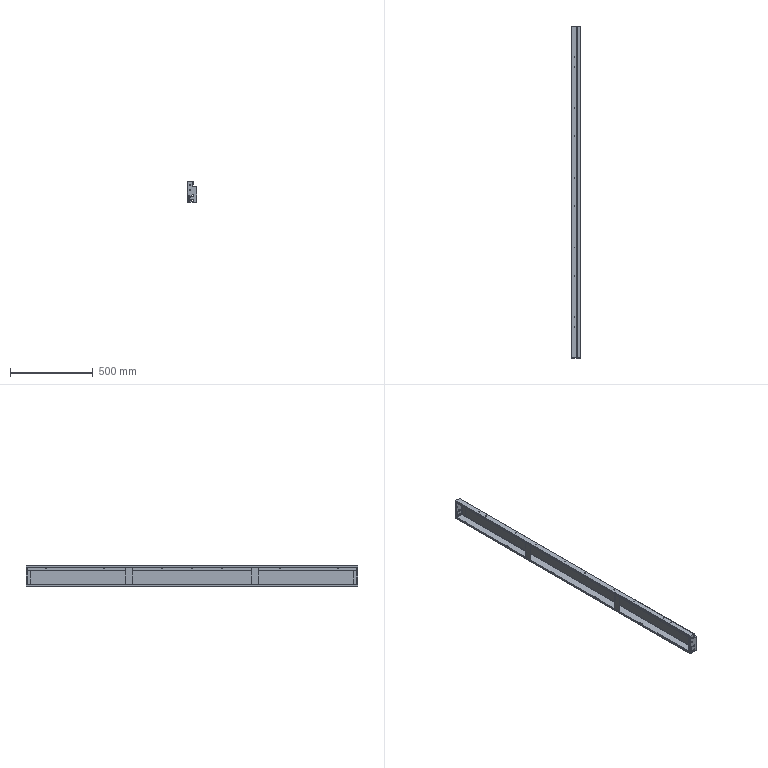Part | 5 solids | 222 faces | box 58 x 2000 x 130 mm | volume 672100 mm3 | plane 122 | cylinder 100 | commonest cylinder face diameters 5 x32 11 x20 9 x18 4.6 x14 2 x10 4.4 x6